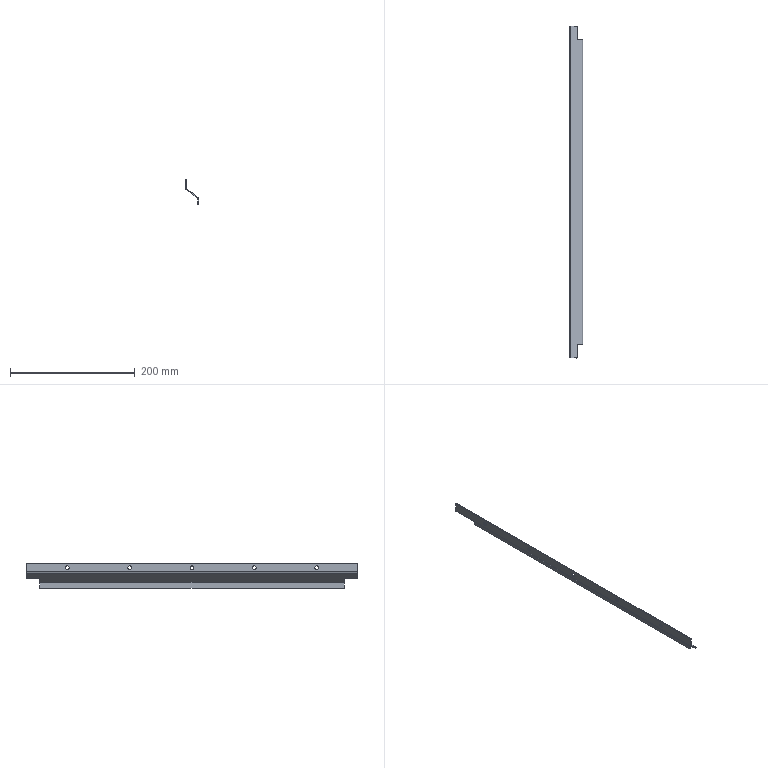Part | NX | features solid 2 | 1 solid | 28 faces | box 21.5 x 533 x 40 mm | volume 38151 mm3 | cylinder 14 | plane 14 | commonest cylinder face diameters 6 x12 3 x2
STEP:
#1=CARTESIAN_POINT('',(-1108.5,-824.5,202.25));
#2=VERTEX_POINT('',#1);
#3=CARTESIAN_POINT('',(-1107.,-824.5,202.25));
#4=VERTEX_POINT('',#3);
#5=CARTESIAN_POINT('',(-1641.931,-824.5,202.25));
#6=DIRECTION('',(1.,0.,0.));
#7=VECTOR('',#6,1000.);
#8=LINE('',#5,#7);
#9=EDGE_CURVE('',#2,#4,#8,.T.);
#10=ORIENTED_EDGE('',*,*,#9,.F.);
#11=CARTESIAN_POINT('',(-1108.5,-824.5,196.25));
#12=VERTEX_POINT('',#11);
#13=CARTESIAN_POINT('',(-1108.5,-824.5,199.25));
#14=DIRECTION('',(1.,0.,0.));
#15=DIRECTION('',(0.,0.,-1.));
#16=AXIS2_PLACEMENT_3D('',#13,#14,#15);
#17=CIRCLE('',#16,3.);
#18=EDGE_CURVE('',#12,#2,#17,.T.);
#19=ORIENTED_EDGE('',*,*,#18,.F.);
#20=CARTESIAN_POINT('',(-1107.,-824.5,196.25));
#21=VERTEX_POINT('',#20);
#22=CARTESIAN_POINT('',(-1641.931,-824.5,196.25));
#23=DIRECTION('',(1.,0.,0.));
#24=VECTOR('',#23,1000.);
#25=LINE('',#22,#24);
#26=EDGE_CURVE('',#21,#12,#25,.F.);
#27=ORIENTED_EDGE('',*,*,#26,.F.);
#28=CARTESIAN_POINT('',(-1107.,-824.5,199.25));
#29=DIRECTION('',(1.,0.,0.));
#30=DIRECTION('',(0.,1.,0.));
#31=AXIS2_PLACEMENT_3D('',#28,#29,#30);
#32=CIRCLE('',#31,3.);
#33=EDGE_CURVE('',#21,#4,#32,.T.);
#34=ORIENTED_EDGE('',*,*,#33,.T.);
#35=EDGE_LOOP('',(#10,#19,#27,#34));
#36=FACE_BOUND('',#35,.T.);
#37=CARTESIAN_POINT('',(-1641.931,-824.5,199.25));
#38=DIRECTION('',(1.,0.,0.));
#39=DIRECTION('',(0.,0.,-1.));
#40=AXIS2_PLACEMENT_3D('',#37,#38,#39);
#41=CYLINDRICAL_SURFACE('',#40,3.);
#42=ADVANCED_FACE('',(#36),#41,.F.);
#43=CARTESIAN_POINT('',(-1108.5,-924.5,202.25));
#44=VERTEX_POINT('',#43);
#45=CARTESIAN_POINT('',(-1107.,-924.5,202.25));
#46=VERTEX_POINT('',#45);
#47=CARTESIAN_POINT('',(-1641.931,-924.5,202.25));
#48=DIRECTION('',(1.,0.,0.));
#49=VECTOR('',#48,1000.);
#50=LINE('',#47,#49);
#51=EDGE_CURVE('',#44,#46,#50,.T.);
#52=ORIENTED_EDGE('',*,*,#51,.F.);
#53=CARTESIAN_POINT('',(-1108.5,-924.5,196.25));
#54=VERTEX_POINT('',#53);
#55=CARTESIAN_POINT('',(-1108.5,-924.5,199.25));
#56=DIRECTION('',(1.,0.,0.));
#57=DIRECTION('',(0.,0.,-1.));
#58=AXIS2_PLACEMENT_3D('',#55,#56,#57);
#59=CIRCLE('',#58,3.);
#60=EDGE_CURVE('',#54,#44,#59,.T.);
#61=ORIENTED_EDGE('',*,*,#60,.F.);
#62=CARTESIAN_POINT('',(-1107.,-924.5,196.25));
#63=VERTEX_POINT('',#62);
#64=CARTESIAN_POINT('',(-1641.931,-924.5,196.25));
#65=DIRECTION('',(1.,0.,0.));
#66=VECTOR('',#65,1000.);
#67=LINE('',#64,#66);
#68=EDGE_CURVE('',#63,#54,#67,.F.);
#69=ORIENTED_EDGE('',*,*,#68,.F.);
#70=CARTESIAN_POINT('',(-1107.,-924.5,199.25));
#71=DIRECTION('',(1.,0.,0.));
#72=DIRECTION('',(0.,1.,0.));
#73=AXIS2_PLACEMENT_3D('',#70,#71,#72);
#74=CIRCLE('',#73,3.);
#75=EDGE_CURVE('',#63,#46,#74,.T.);
#76=ORIENTED_EDGE('',*,*,#75,.T.);
#77=EDGE_LOOP('',(#52,#61,#69,#76));
#78=FACE_BOUND('',#77,.T.);
#79=CARTESIAN_POINT('',(-1641.931,-924.5,199.25));
#80=DIRECTION('',(1.,0.,0.));
#81=DIRECTION('',(0.,0.,-1.));
#82=AXIS2_PLACEMENT_3D('',#79,#80,#81);
#83=CYLINDRICAL_SURFACE('',#82,3.);
#84=ADVANCED_FACE('',(#78),#83,.F.);
#85=CARTESIAN_POINT('',(-1108.5,-1024.5,202.25));
#86=VERTEX_POINT('',#85);
#87=CARTESIAN_POINT('',(-1107.,-1024.5,202.25));
#88=VERTEX_POINT('',#87);
#89=CARTESIAN_POINT('',(-1641.931,-1024.5,202.25));
#90=DIRECTION('',(1.,0.,0.));
#91=VECTOR('',#90,1000.);
#92=LINE('',#89,#91);
#93=EDGE_CURVE('',#86,#88,#92,.T.);
#94=ORIENTED_EDGE('',*,*,#93,.F.);
#95=CARTESIAN_POINT('',(-1108.5,-1024.5,196.25));
#96=VERTEX_POINT('',#95);
#97=CARTESIAN_POINT('',(-1108.5,-1024.5,199.25));
#98=DIRECTION('',(1.,0.,0.));
#99=DIRECTION('',(0.,0.,-1.));
#100=AXIS2_PLACEMENT_3D('',#97,#98,#99);
#101=CIRCLE('',#100,3.);
#102=EDGE_CURVE('',#96,#86,#101,.T.);
#103=ORIENTED_EDGE('',*,*,#102,.F.);
#104=CARTESIAN_POINT('',(-1107.,-1024.5,196.25));
#105=VERTEX_POINT('',#104);
#106=CARTESIAN_POINT('',(-1641.931,-1024.5,196.25));
#107=DIRECTION('',(1.,0.,0.));
#108=VECTOR('',#107,1000.);
#109=LINE('',#106,#108);
#110=EDGE_CURVE('',#105,#96,#109,.F.);
#111=ORIENTED_EDGE('',*,*,#110,.F.);
#112=CARTESIAN_POINT('',(-1107.,-1024.5,199.25));
#113=DIRECTION('',(1.,0.,0.));
#114=DIRECTION('',(0.,1.,0.));
#115=AXIS2_PLACEMENT_3D('',#112,#113,#114);
#116=CIRCLE('',#115,3.);
#117=EDGE_CURVE('',#105,#88,#116,.T.);
#118=ORIENTED_EDGE('',*,*,#117,.T.);
#119=EDGE_LOOP('',(#94,#103,#111,#118));
#120=FACE_BOUND('',#119,.T.);
#121=CARTESIAN_POINT('',(-1641.931,-1024.5,199.25));
#122=DIRECTION('',(1.,0.,0.));
#123=DIRECTION('',(0.,0.,-1.));
#124=AXIS2_PLACEMENT_3D('',#121,#122,#123);
#125=CYLINDRICAL_SURFACE('',#124,3.);
#126=ADVANCED_FACE('',(#120),#125,.F.);
#127=CARTESIAN_POINT('',(-1107.,-1124.5,202.25));
#128=VERTEX_POINT('',#127);
#129=CARTESIAN_POINT('',(-1108.5,-1124.5,202.25));
#130=VERTEX_POINT('',#129);
#131=CARTESIAN_POINT('',(-1641.931,-1124.5,202.25));
#132=DIRECTION('',(1.,0.,0.));
#133=VECTOR('',#132,1000.);
#134=LINE('',#131,#133);
#135=EDGE_CURVE('',#128,#130,#134,.F.);
#136=ORIENTED_EDGE('',*,*,#135,.T.);
#137=CARTESIAN_POINT('',(-1108.5,-1124.5,196.25));
#138=VERTEX_POINT('',#137);
#139=CARTESIAN_POINT('',(-1108.5,-1124.5,199.25));
#140=DIRECTION('',(1.,0.,0.));
#141=DIRECTION('',(0.,0.,-1.));
#142=AXIS2_PLACEMENT_3D('',#139,#140,#141);
#143=CIRCLE('',#142,3.);
#144=EDGE_CURVE('',#138,#130,#143,.T.);
#145=ORIENTED_EDGE('',*,*,#144,.F.);
#146=CARTESIAN_POINT('',(-1107.,-1124.5,196.25));
#147=VERTEX_POINT('',#146);
#148=CARTESIAN_POINT('',(-1641.931,-1124.5,196.25));
#149=DIRECTION('',(1.,0.,0.));
#150=VECTOR('',#149,1000.);
#151=LINE('',#148,#150);
#152=EDGE_CURVE('',#138,#147,#151,.T.);
#153=ORIENTED_EDGE('',*,*,#152,.T.);
#154=CARTESIAN_POINT('',(-1107.,-1124.5,199.25));
#155=DIRECTION('',(1.,0.,0.));
#156=DIRECTION('',(0.,1.,0.));
#157=AXIS2_PLACEMENT_3D('',#154,#155,#156);
#158=CIRCLE('',#157,3.);
#159=EDGE_CURVE('',#147,#128,#158,.T.);
#160=ORIENTED_EDGE('',*,*,#159,.T.);
#161=EDGE_LOOP('',(#136,#145,#153,#160));
#162=FACE_BOUND('',#161,.T.);
#163=CARTESIAN_POINT('',(-1641.931,-1124.5,199.25));
#164=DIRECTION('',(1.,0.,0.));
#165=DIRECTION('',(0.,0.,-1.));
#166=AXIS2_PLACEMENT_3D('',#163,#164,#165);
#167=CYLINDRICAL_SURFACE('',#166,3.);
#168=ADVANCED_FACE('',(#162),#167,.F.);
#169=CARTESIAN_POINT('',(-1108.5,-1224.5,202.25));
#170=VERTEX_POINT('',#169);
#171=CARTESIAN_POINT('',(-1107.,-1224.5,202.25));
#172=VERTEX_POINT('',#171);
#173=CARTESIAN_POINT('',(-1641.931,-1224.5,202.25));
#174=DIRECTION('',(1.,0.,0.));
#175=VECTOR('',#174,1000.);
#176=LINE('',#173,#175);
#177=EDGE_CURVE('',#170,#172,#176,.T.);
#178=ORIENTED_EDGE('',*,*,#177,.F.);
#179=CARTESIAN_POINT('',(-1108.5,-1224.5,196.25));
#180=VERTEX_POINT('',#179);
#181=CARTESIAN_POINT('',(-1108.5,-1224.5,199.25));
#182=DIRECTION('',(1.,0.,0.));
#183=DIRECTION('',(0.,0.,-1.));
#184=AXIS2_PLACEMENT_3D('',#181,#182,#183);
#185=CIRCLE('',#184,3.);
#186=EDGE_CURVE('',#180,#170,#185,.T.);
#187=ORIENTED_EDGE('',*,*,#186,.F.);
#188=CARTESIAN_POINT('',(-1107.,-1224.5,196.25));
#189=VERTEX_POINT('',#188);
#190=CARTESIAN_POINT('',(-1641.931,-1224.5,196.25));
#191=DIRECTION('',(1.,0.,0.));
#192=VECTOR('',#191,1000.);
#193=LINE('',#190,#192);
#194=EDGE_CURVE('',#189,#180,#193,.F.);
#195=ORIENTED_EDGE('',*,*,#194,.F.);
#196=CARTESIAN_POINT('',(-1107.,-1224.5,199.25));
#197=DIRECTION('',(1.,0.,0.));
#198=DIRECTION('',(0.,1.,0.));
#199=AXIS2_PLACEMENT_3D('',#196,#197,#198);
#200=CIRCLE('',#199,3.);
#201=EDGE_CURVE('',#189,#172,#200,.T.);
#202=ORIENTED_EDGE('',*,*,#201,.T.);
#203=EDGE_LOOP('',(#178,#187,#195,#202));
#204=FACE_BOUND('',#203,.T.);
#205=CARTESIAN_POINT('',(-1641.931,-1224.5,199.25));
#206=DIRECTION('',(1.,0.,0.));
#207=DIRECTION('',(0.,0.,-1.));
#208=AXIS2_PLACEMENT_3D('',#205,#206,#207);
#209=CYLINDRICAL_SURFACE('',#208,3.);
#210=ADVANCED_FACE('',(#204),#209,.F.);
#211=CARTESIAN_POINT('',(-1088.5,-1269.,166.));
#212=VERTEX_POINT('',#211);
#213=CARTESIAN_POINT('',(-1087.,-1269.,166.));
#214=VERTEX_POINT('',#213);
#215=CARTESIAN_POINT('',(-1087.,-1269.,166.));
#216=DIRECTION('',(1.,0.,0.));
#217=VECTOR('',#216,1000.);
#218=LINE('',#215,#217);
#219=EDGE_CURVE('',#212,#214,#218,.T.);
#220=ORIENTED_EDGE('',*,*,#219,.T.);
#221=CARTESIAN_POINT('',(-1087.,-1269.,175.25));
#222=VERTEX_POINT('',#221);
#223=CARTESIAN_POINT('',(-1087.,-1269.,176.));
#224=DIRECTION('',(0.,0.,1.));
#225=VECTOR('',#224,1000.);
#226=LINE('',#223,#225);
#227=EDGE_CURVE('',#214,#222,#226,.T.);
#228=ORIENTED_EDGE('',*,*,#227,.T.);
#229=CARTESIAN_POINT('',(-1088.2,-1269.,177.65));
#230=VERTEX_POINT('',#229);
#231=CARTESIAN_POINT('',(-1090.,-1269.,175.25));
#232=DIRECTION('',(0.,-1.,0.));
#233=DIRECTION('',(0.,0.,-1.));
#234=AXIS2_PLACEMENT_3D('',#231,#232,#233);
#235=CIRCLE('',#234,3.);
#236=EDGE_CURVE('',#222,#230,#235,.T.);
#237=ORIENTED_EDGE('',*,*,#236,.T.);
#238=CARTESIAN_POINT('',(-1095.5,-1269.,183.125));
#239=VERTEX_POINT('',#238);
#240=CARTESIAN_POINT('',(-1107.6,-1269.,192.2));
#241=DIRECTION('',(-0.8,0.,0.6));
#242=VECTOR('',#241,1000.);
#243=LINE('',#240,#242);
#244=EDGE_CURVE('',#230,#239,#243,.T.);
#245=ORIENTED_EDGE('',*,*,#244,.T.);
#246=CARTESIAN_POINT('',(-1096.4,-1269.,181.925));
#247=VERTEX_POINT('',#246);
#248=CARTESIAN_POINT('',(-1095.5,-1269.,183.125));
#249=DIRECTION('',(0.6,0.,0.8));
#250=VECTOR('',#249,1000.);
#251=LINE('',#248,#250);
#252=EDGE_CURVE('',#247,#239,#251,.T.);
#253=ORIENTED_EDGE('',*,*,#252,.F.);
#254=CARTESIAN_POINT('',(-1089.1,-1269.,176.45));
#255=VERTEX_POINT('',#254);
#256=CARTESIAN_POINT('',(-1108.5,-1269.,191.));
#257=DIRECTION('',(-0.8,0.,0.6));
#258=VECTOR('',#257,1000.);
#259=LINE('',#256,#258);
#260=EDGE_CURVE('',#255,#247,#259,.T.);
#261=ORIENTED_EDGE('',*,*,#260,.F.);
#262=CARTESIAN_POINT('',(-1088.5,-1269.,175.25));
#263=VERTEX_POINT('',#262);
#264=CARTESIAN_POINT('',(-1090.,-1269.,175.25));
#265=DIRECTION('',(0.,-1.,0.));
#266=DIRECTION('',(0.,0.,-1.));
#267=AXIS2_PLACEMENT_3D('',#264,#265,#266);
#268=CIRCLE('',#267,1.5);
#269=EDGE_CURVE('',#263,#255,#268,.T.);
#270=ORIENTED_EDGE('',*,*,#269,.F.);
#271=CARTESIAN_POINT('',(-1088.5,-1269.,176.));
#272=DIRECTION('',(0.,0.,1.));
#273=VECTOR('',#272,1000.);
#274=LINE('',#271,#273);
#275=EDGE_CURVE('',#212,#263,#274,.T.);
#276=ORIENTED_EDGE('',*,*,#275,.F.);
#277=EDGE_LOOP('',(#220,#228,#237,#245,#253,#261,#270,#276));
#278=FACE_BOUND('',#277,.T.);
#279=CARTESIAN_POINT('',(-1087.,-1269.,176.));
#280=DIRECTION('',(0.,1.,0.));
#281=DIRECTION('',(1.,0.,0.));
#282=AXIS2_PLACEMENT_3D('',#279,#280,#281);
#283=PLANE('',#282);
#284=ADVANCED_FACE('',(#278),#283,.F.);
#285=ORIENTED_EDGE('',*,*,#252,.T.);
#286=CARTESIAN_POINT('',(-1095.5,-1291.,183.125));
#287=VERTEX_POINT('',#286);
#288=CARTESIAN_POINT('',(-1095.5,-1291.,183.125));
#289=DIRECTION('',(0.,-1.,0.));
#290=VECTOR('',#289,1000.);
#291=LINE('',#288,#290);
#292=EDGE_CURVE('',#239,#287,#291,.T.);
#293=ORIENTED_EDGE('',*,*,#292,.T.);
#294=CARTESIAN_POINT('',(-1096.4,-1291.,181.925));
#295=VERTEX_POINT('',#294);
#296=CARTESIAN_POINT('',(-1095.5,-1291.,183.125));
#297=DIRECTION('',(0.6,0.,0.8));
#298=VECTOR('',#297,1000.);
#299=LINE('',#296,#298);
#300=EDGE_CURVE('',#295,#287,#299,.T.);
#301=ORIENTED_EDGE('',*,*,#300,.F.);
#302=CARTESIAN_POINT('',(-1096.4,-1291.,181.925));
#303=DIRECTION('',(0.,-1.,0.));
#304=VECTOR('',#303,1000.);
#305=LINE('',#302,#304);
#306=EDGE_CURVE('',#247,#295,#305,.T.);
#307=ORIENTED_EDGE('',*,*,#306,.F.);
#308=EDGE_LOOP('',(#285,#293,#301,#307));
#309=FACE_BOUND('',#308,.T.);
#310=CARTESIAN_POINT('',(-1095.5,-1291.,183.125));
#311=DIRECTION('',(-0.8,0.,0.6));
#312=DIRECTION('',(0.,1.,0.));
#313=AXIS2_PLACEMENT_3D('',#310,#311,#312);
#314=PLANE('',#313);
#315=ADVANCED_FACE('',(#309),#314,.F.);
#316=CARTESIAN_POINT('',(-1088.5,-780.,175.25));
#317=VERTEX_POINT('',#316);
#318=CARTESIAN_POINT('',(-1088.5,-780.,166.));
#319=VERTEX_POINT('',#318);
#320=CARTESIAN_POINT('',(-1088.5,-780.,176.));
#321=DIRECTION('',(0.,0.,-1.));
#322=VECTOR('',#321,1000.);
#323=LINE('',#320,#322);
#324=EDGE_CURVE('',#317,#319,#323,.T.);
#325=ORIENTED_EDGE('',*,*,#324,.F.);
#326=CARTESIAN_POINT('',(-1089.1,-780.,176.45));
#327=VERTEX_POINT('',#326);
#328=CARTESIAN_POINT('',(-1090.,-780.,175.25));
#329=DIRECTION('',(0.,1.,0.));
#330=DIRECTION('',(0.,0.,-1.));
#331=AXIS2_PLACEMENT_3D('',#328,#329,#330);
#332=CIRCLE('',#331,1.5);
#333=EDGE_CURVE('',#327,#317,#332,.T.);
#334=ORIENTED_EDGE('',*,*,#333,.F.);
#335=CARTESIAN_POINT('',(-1096.4,-780.,181.925));
#336=VERTEX_POINT('',#335);
#337=CARTESIAN_POINT('',(-1108.5,-780.,191.));
#338=DIRECTION('',(0.8,0.,-0.6));
#339=VECTOR('',#338,1000.);
#340=LINE('',#337,#339);
#341=EDGE_CURVE('',#336,#327,#340,.T.);
#342=ORIENTED_EDGE('',*,*,#341,.F.);
#343=CARTESIAN_POINT('',(-1095.5,-780.,183.125));
#344=VERTEX_POINT('',#343);
#345=CARTESIAN_POINT('',(-1095.5,-780.,183.125));
#346=DIRECTION('',(0.6,0.,0.8));
#347=VECTOR('',#346,1000.);
#348=LINE('',#345,#347);
#349=EDGE_CURVE('',#336,#344,#348,.T.);
#350=ORIENTED_EDGE('',*,*,#349,.T.);
#351=CARTESIAN_POINT('',(-1088.2,-780.,177.65));
#352=VERTEX_POINT('',#351);
#353=CARTESIAN_POINT('',(-1107.6,-780.,192.2));
#354=DIRECTION('',(0.8,0.,-0.6));
#355=VECTOR('',#354,1000.);
#356=LINE('',#353,#355);
#357=EDGE_CURVE('',#344,#352,#356,.T.);
#358=ORIENTED_EDGE('',*,*,#357,.T.);
#359=CARTESIAN_POINT('',(-1087.,-780.,175.25));
#360=VERTEX_POINT('',#359);
#361=CARTESIAN_POINT('',(-1090.,-780.,175.25));
#362=DIRECTION('',(0.,1.,0.));
#363=DIRECTION('',(0.,0.,1.));
#364=AXIS2_PLACEMENT_3D('',#361,#362,#363);
#365=CIRCLE('',#364,3.);
#366=EDGE_CURVE('',#352,#360,#365,.T.);
#367=ORIENTED_EDGE('',*,*,#366,.T.);
#368=CARTESIAN_POINT('',(-1087.,-780.,166.));
#369=VERTEX_POINT('',#368);
#370=CARTESIAN_POINT('',(-1087.,-780.,176.));
#371=DIRECTION('',(0.,0.,-1.));
#372=VECTOR('',#371,1000.);
#373=LINE('',#370,#372);
#374=EDGE_CURVE('',#360,#369,#373,.T.);
#375=ORIENTED_EDGE('',*,*,#374,.T.);
#376=CARTESIAN_POINT('',(-1087.,-780.,166.));
#377=DIRECTION('',(1.,0.,0.));
#378=VECTOR('',#377,1000.);
#379=LINE('',#376,#378);
#380=EDGE_CURVE('',#319,#369,#379,.T.);
#381=ORIENTED_EDGE('',*,*,#380,.F.);
#382=EDGE_LOOP('',(#325,#334,#342,#350,#358,#367,#375,#381));
#383=FACE_BOUND('',#382,.T.);
#384=CARTESIAN_POINT('',(-1087.,-780.,176.));
#385=DIRECTION('',(0.,-1.,0.));
#386=DIRECTION('',(-1.,0.,0.));
#387=AXIS2_PLACEMENT_3D('',#384,#385,#386);
#388=PLANE('',#387);
#389=ADVANCED_FACE('',(#383),#388,.F.);
#390=CARTESIAN_POINT('',(-1096.4,-758.,181.925));
#391=VERTEX_POINT('',#390);
#392=CARTESIAN_POINT('',(-1095.5,-758.,183.125));
#393=VERTEX_POINT('',#392);
#394=CARTESIAN_POINT('',(-1095.5,-758.,183.125));
#395=DIRECTION('',(0.6,0.,0.8));
#396=VECTOR('',#395,1000.);
#397=LINE('',#394,#396);
#398=EDGE_CURVE('',#391,#393,#397,.T.);
#399=ORIENTED_EDGE('',*,*,#398,.T.);
#400=CARTESIAN_POINT('',(-1095.5,-1291.,183.125));
#401=DIRECTION('',(0.,-1.,0.));
#402=VECTOR('',#401,1000.);
#403=LINE('',#400,#402);
#404=EDGE_CURVE('',#393,#344,#403,.T.);
#405=ORIENTED_EDGE('',*,*,#404,.T.);
#406=ORIENTED_EDGE('',*,*,#349,.F.);
#407=CARTESIAN_POINT('',(-1096.4,-1291.,181.925));
#408=DIRECTION('',(0.,-1.,0.));
#409=VECTOR('',#408,1000.);
#410=LINE('',#407,#409);
#411=EDGE_CURVE('',#391,#336,#410,.T.);
#412=ORIENTED_EDGE('',*,*,#411,.F.);
#413=EDGE_LOOP('',(#399,#405,#406,#412));
#414=FACE_BOUND('',#413,.T.);
#415=CARTESIAN_POINT('',(-1095.5,-1291.,183.125));
#416=DIRECTION('',(-0.8,0.,0.6));
#417=DIRECTION('',(0.,1.,0.));
#418=AXIS2_PLACEMENT_3D('',#415,#416,#417);
#419=PLANE('',#418);
#420=ADVANCED_FACE('',(#414),#419,.F.);
#421=CARTESIAN_POINT('',(-1088.5,-1291.,166.));
#422=DIRECTION('',(0.,1.,0.));
#423=VECTOR('',#422,1000.);
#424=LINE('',#421,#423);
#425=EDGE_CURVE('',#212,#319,#424,.T.);
#426=ORIENTED_EDGE('',*,*,#425,.F.);
#427=ORIENTED_EDGE('',*,*,#275,.T.);
#428=CARTESIAN_POINT('',(-1088.5,-1291.,175.25));
#429=DIRECTION('',(0.,1.,0.));
#430=VECTOR('',#429,1000.);
#431=LINE('',#428,#430);
#432=EDGE_CURVE('',#263,#317,#431,.T.);
#433=ORIENTED_EDGE('',*,*,#432,.T.);
#434=ORIENTED_EDGE('',*,*,#324,.T.);
#435=EDGE_LOOP('',(#426,#427,#433,#434));
#436=FACE_BOUND('',#435,.T.);
#437=CARTESIAN_POINT('',(-1088.5,-1291.,176.));
#438=DIRECTION('',(1.,0.,0.));
#439=DIRECTION('',(0.,0.,-1.));
#440=AXIS2_PLACEMENT_3D('',#437,#438,#439);
#441=PLANE('',#440);
#442=ADVANCED_FACE('',(#436),#441,.F.);
#443=ORIENTED_EDGE('',*,*,#432,.F.);
#444=ORIENTED_EDGE('',*,*,#269,.T.);
#445=CARTESIAN_POINT('',(-1089.1,-1291.,176.45));
#446=DIRECTION('',(0.,1.,0.));
#447=VECTOR('',#446,1000.);
#448=LINE('',#445,#447);
#449=EDGE_CURVE('',#255,#327,#448,.T.);
#450=ORIENTED_EDGE('',*,*,#449,.T.);
#451=ORIENTED_EDGE('',*,*,#333,.T.);
#452=EDGE_LOOP('',(#443,#444,#450,#451));
#453=FACE_BOUND('',#452,.T.);
#454=CARTESIAN_POINT('',(-1090.,-1291.,175.25));
#455=DIRECTION('',(0.,1.,0.));
#456=DIRECTION('',(0.,0.,-1.));
#457=AXIS2_PLACEMENT_3D('',#454,#455,#456);
#458=CYLINDRICAL_SURFACE('',#457,1.5);
#459=ADVANCED_FACE('',(#453),#458,.F.);
#460=ORIENTED_EDGE('',*,*,#260,.T.);
#461=ORIENTED_EDGE('',*,*,#306,.T.);
#462=CARTESIAN_POINT('',(-1107.3,-1291.,190.1));
#463=VERTEX_POINT('',#462);
#464=CARTESIAN_POINT('',(-1108.5,-1291.,191.));
#465=DIRECTION('',(0.8,0.,-0.6));
#466=VECTOR('',#465,1000.);
#467=LINE('',#464,#466);
#468=EDGE_CURVE('',#463,#295,#467,.T.);
#469=ORIENTED_EDGE('',*,*,#468,.F.);
#470=CARTESIAN_POINT('',(-1107.3,-758.,190.1));
#471=VERTEX_POINT('',#470);
#472=CARTESIAN_POINT('',(-1107.3,-1291.,190.1));
#473=DIRECTION('',(0.,1.,0.));
#474=VECTOR('',#473,1000.);
#475=LINE('',#472,#474);
#476=EDGE_CURVE('',#463,#471,#475,.T.);
#477=ORIENTED_EDGE('',*,*,#476,.T.);
#478=CARTESIAN_POINT('',(-1108.5,-758.,191.));
#479=DIRECTION('',(0.8,0.,-0.6));
#480=VECTOR('',#479,1000.);
#481=LINE('',#478,#480);
#482=EDGE_CURVE('',#471,#391,#481,.T.);
#483=ORIENTED_EDGE('',*,*,#482,.T.);
#484=ORIENTED_EDGE('',*,*,#411,.T.);
#485=ORIENTED_EDGE('',*,*,#341,.T.);
#486=ORIENTED_EDGE('',*,*,#449,.F.);
#487=EDGE_LOOP('',(#460,#461,#469,#477,#483,#484,#485,#486));
#488=FACE_BOUND('',#487,.T.);
#489=CARTESIAN_POINT('',(-1108.5,-1291.,191.));
#490=DIRECTION('',(0.6,0.,0.8));
#491=DIRECTION('',(0.,-1.,0.));
#492=AXIS2_PLACEMENT_3D('',#489,#490,#491);
#493=PLANE('',#492);
#494=ADVANCED_FACE('',(#488),#493,.F.);
#495=CARTESIAN_POINT('',(-1108.5,-758.,192.5));
#496=VERTEX_POINT('',#495);
#497=CARTESIAN_POINT('',(-1105.5,-758.,192.5));
#498=DIRECTION('',(0.,-1.,0.));
#499=DIRECTION('',(0.,0.,-1.));
#500=AXIS2_PLACEMENT_3D('',#497,#498,#499);
#501=CIRCLE('',#500,3.);
#502=EDGE_CURVE('',#496,#471,#501,.T.);
#503=ORIENTED_EDGE('',*,*,#502,.T.);
#504=ORIENTED_EDGE('',*,*,#476,.F.);
#505=CARTESIAN_POINT('',(-1108.5,-1291.,192.5));
#506=VERTEX_POINT('',#505);
#507=CARTESIAN_POINT('',(-1105.5,-1291.,192.5));
#508=DIRECTION('',(0.,-1.,0.));
#509=DIRECTION('',(0.,0.,-1.));
#510=AXIS2_PLACEMENT_3D('',#507,#508,#509);
#511=CIRCLE('',#510,3.);
#512=EDGE_CURVE('',#506,#463,#511,.T.);
#513=ORIENTED_EDGE('',*,*,#512,.F.);
#514=CARTESIAN_POINT('',(-1108.5,-1291.,192.5));
#515=DIRECTION('',(0.,1.,0.));
#516=VECTOR('',#515,1000.);
#517=LINE('',#514,#516);
#518=EDGE_CURVE('',#506,#496,#517,.T.);
#519=ORIENTED_EDGE('',*,*,#518,.T.);
#520=EDGE_LOOP('',(#503,#504,#513,#519));
#521=FACE_BOUND('',#520,.T.);
#522=CARTESIAN_POINT('',(-1105.5,-1291.,192.5));
#523=DIRECTION('',(0.,1.,0.));
#524=DIRECTION('',(0.,0.,-1.));
#525=AXIS2_PLACEMENT_3D('',#522,#523,#524);
#526=CYLINDRICAL_SURFACE('',#525,3.);
#527=ADVANCED_FACE('',(#521),#526,.T.);
#528=ORIENTED_EDGE('',*,*,#186,.T.);
#529=CARTESIAN_POINT('',(-1108.5,-1224.5,199.25));
#530=DIRECTION('',(1.,0.,0.));
#531=DIRECTION('',(0.,0.,-1.));
#532=AXIS2_PLACEMENT_3D('',#529,#530,#531);
#533=CIRCLE('',#532,3.);
#534=EDGE_CURVE('',#170,#180,#533,.T.);
#535=ORIENTED_EDGE('',*,*,#534,.T.);
#536=EDGE_LOOP('',(#528,#535));
#537=FACE_BOUND('',#536,.T.);
#538=ORIENTED_EDGE('',*,*,#144,.T.);
#539=CARTESIAN_POINT('',(-1108.5,-1124.5,199.25));
#540=DIRECTION('',(1.,0.,0.));
#541=DIRECTION('',(0.,0.,-1.));
#542=AXIS2_PLACEMENT_3D('',#539,#540,#541);
#543=CIRCLE('',#542,3.);
#544=EDGE_CURVE('',#130,#138,#543,.T.);
#545=ORIENTED_EDGE('',*,*,#544,.T.);
#546=EDGE_LOOP('',(#538,#545));
#547=FACE_BOUND('',#546,.T.);
#548=ORIENTED_EDGE('',*,*,#102,.T.);
#549=CARTESIAN_POINT('',(-1108.5,-1024.5,199.25));
#550=DIRECTION('',(1.,0.,0.));
#551=DIRECTION('',(0.,0.,-1.));
#552=AXIS2_PLACEMENT_3D('',#549,#550,#551);
#553=CIRCLE('',#552,3.);
#554=EDGE_CURVE('',#86,#96,#553,.T.);
#555=ORIENTED_EDGE('',*,*,#554,.T.);
#556=EDGE_LOOP('',(#548,#555));
#557=FACE_BOUND('',#556,.T.);
#558=ORIENTED_EDGE('',*,*,#60,.T.);
#559=CARTESIAN_POINT('',(-1108.5,-924.5,199.25));
#560=DIRECTION('',(1.,0.,0.));
#561=DIRECTION('',(0.,0.,-1.));
#562=AXIS2_PLACEMENT_3D('',#559,#560,#561);
#563=CIRCLE('',#562,3.);
#564=EDGE_CURVE('',#44,#54,#563,.T.);
#565=ORIENTED_EDGE('',*,*,#564,.T.);
#566=EDGE_LOOP('',(#558,#565));
#567=FACE_BOUND('',#566,.T.);
#568=ORIENTED_EDGE('',*,*,#18,.T.);
#569=CARTESIAN_POINT('',(-1108.5,-824.5,199.25));
#570=DIRECTION('',(1.,0.,0.));
#571=DIRECTION('',(0.,0.,-1.));
#572=AXIS2_PLACEMENT_3D('',#569,#570,#571);
#573=CIRCLE('',#572,3.);
#574=EDGE_CURVE('',#2,#12,#573,.T.);
#575=ORIENTED_EDGE('',*,*,#574,.T.);
#576=EDGE_LOOP('',(#568,#575));
#577=FACE_BOUND('',#576,.T.);
#578=CARTESIAN_POINT('',(-1108.5,-758.,206.));
#579=VERTEX_POINT('',#578);
#580=CARTESIAN_POINT('',(-1108.5,-758.,191.));
#581=DIRECTION('',(0.,0.,-1.));
#582=VECTOR('',#581,1000.);
#583=LINE('',#580,#582);
#584=EDGE_CURVE('',#579,#496,#583,.T.);
#585=ORIENTED_EDGE('',*,*,#584,.T.);
#586=ORIENTED_EDGE('',*,*,#518,.F.);
#587=CARTESIAN_POINT('',(-1108.5,-1291.,206.));
#588=VERTEX_POINT('',#587);
#589=CARTESIAN_POINT('',(-1108.5,-1291.,191.));
#590=DIRECTION('',(0.,0.,-1.));
#591=VECTOR('',#590,1000.);
#592=LINE('',#589,#591);
#593=EDGE_CURVE('',#588,#506,#592,.T.);
#594=ORIENTED_EDGE('',*,*,#593,.F.);
#595=CARTESIAN_POINT('',(-1108.5,-1291.,206.));
#596=DIRECTION('',(0.,1.,0.));
#597=VECTOR('',#596,1000.);
#598=LINE('',#595,#597);
#599=EDGE_CURVE('',#588,#579,#598,.T.);
#600=ORIENTED_EDGE('',*,*,#599,.T.);
#601=EDGE_LOOP('',(#585,#586,#594,#600));
#602=FACE_BOUND('',#601,.T.);
#603=CARTESIAN_POINT('',(-1108.5,-1291.,191.));
#604=DIRECTION('',(1.,0.,0.));
#605=DIRECTION('',(0.,0.,-1.));
#606=AXIS2_PLACEMENT_3D('',#603,#604,#605);
#607=PLANE('',#606);
#608=ADVANCED_FACE('',(#537,#547,#557,#567,#577,#602),#607,.F.);
#609=ORIENTED_EDGE('',*,*,#227,.F.);
#610=CARTESIAN_POINT('',(-1087.,-1291.,166.));
#611=DIRECTION('',(0.,1.,0.));
#612=VECTOR('',#611,1000.);
#613=LINE('',#610,#612);
#614=EDGE_CURVE('',#214,#369,#613,.T.);
#615=ORIENTED_EDGE('',*,*,#614,.T.);
#616=ORIENTED_EDGE('',*,*,#374,.F.);
#617=CARTESIAN_POINT('',(-1087.,-1291.,175.25));
#618=DIRECTION('',(0.,1.,0.));
#619=VECTOR('',#618,1000.);
#620=LINE('',#617,#619);
#621=EDGE_CURVE('',#222,#360,#620,.T.);
#622=ORIENTED_EDGE('',*,*,#621,.F.);
#623=EDGE_LOOP('',(#609,#615,#616,#622));
#624=FACE_BOUND('',#623,.T.);
#625=CARTESIAN_POINT('',(-1087.,-1291.,176.));
#626=DIRECTION('',(1.,0.,0.));
#627=DIRECTION('',(0.,0.,-1.));
#628=AXIS2_PLACEMENT_3D('',#625,#626,#627);
#629=PLANE('',#628);
#630=ADVANCED_FACE('',(#624),#629,.T.);
#631=ORIENTED_EDGE('',*,*,#236,.F.);
#632=ORIENTED_EDGE('',*,*,#621,.T.);
#633=ORIENTED_EDGE('',*,*,#366,.F.);
#634=CARTESIAN_POINT('',(-1088.2,-1291.,177.65));
#635=DIRECTION('',(0.,1.,0.));
#636=VECTOR('',#635,1000.);
#637=LINE('',#634,#636);
#638=EDGE_CURVE('',#230,#352,#637,.T.);
#639=ORIENTED_EDGE('',*,*,#638,.F.);
#640=EDGE_LOOP('',(#631,#632,#633,#639));
#641=FACE_BOUND('',#640,.T.);
#642=CARTESIAN_POINT('',(-1090.,-1291.,175.25));
#643=DIRECTION('',(0.,1.,0.));
#644=DIRECTION('',(0.,0.,-1.));
#645=AXIS2_PLACEMENT_3D('',#642,#643,#644);
#646=CYLINDRICAL_SURFACE('',#645,3.);
#647=ADVANCED_FACE('',(#641),#646,.T.);
#648=ORIENTED_EDGE('',*,*,#292,.F.);
#649=ORIENTED_EDGE('',*,*,#244,.F.);
#650=ORIENTED_EDGE('',*,*,#638,.T.);
#651=ORIENTED_EDGE('',*,*,#357,.F.);
#652=ORIENTED_EDGE('',*,*,#404,.F.);
#653=CARTESIAN_POINT('',(-1106.4,-758.,191.3));
#654=VERTEX_POINT('',#653);
#655=CARTESIAN_POINT('',(-1107.6,-758.,192.2));
#656=DIRECTION('',(0.8,0.,-0.6));
#657=VECTOR('',#656,1000.);
#658=LINE('',#655,#657);
#659=EDGE_CURVE('',#654,#393,#658,.T.);
#660=ORIENTED_EDGE('',*,*,#659,.F.);
#661=CARTESIAN_POINT('',(-1106.4,-1291.,191.3));
#662=VERTEX_POINT('',#661);
#663=CARTESIAN_POINT('',(-1106.4,-1291.,191.3));
#664=DIRECTION('',(0.,1.,0.));
#665=VECTOR('',#664,1000.);
#666=LINE('',#663,#665);
#667=EDGE_CURVE('',#662,#654,#666,.T.);
#668=ORIENTED_EDGE('',*,*,#667,.F.);
#669=CARTESIAN_POINT('',(-1107.6,-1291.,192.2));
#670=DIRECTION('',(0.8,0.,-0.6));
#671=VECTOR('',#670,1000.);
#672=LINE('',#669,#671);
#673=EDGE_CURVE('',#662,#287,#672,.T.);
#674=ORIENTED_EDGE('',*,*,#673,.T.);
#675=EDGE_LOOP('',(#648,#649,#650,#651,#652,#660,#668,#674));
#676=FACE_BOUND('',#675,.T.);
#677=CARTESIAN_POINT('',(-1107.6,-1291.,192.2));
#678=DIRECTION('',(0.6,0.,0.8));
#679=DIRECTION('',(0.,-1.,0.));
#680=AXIS2_PLACEMENT_3D('',#677,#678,#679);
#681=PLANE('',#680);
#682=ADVANCED_FACE('',(#676),#681,.T.);
#683=CARTESIAN_POINT('',(-1107.,-758.,192.5));
#684=VERTEX_POINT('',#683);
#685=CARTESIAN_POINT('',(-1105.5,-758.,192.5));
#686=DIRECTION('',(0.,-1.,0.));
#687=DIRECTION('',(0.,0.,-1.));
#688=AXIS2_PLACEMENT_3D('',#685,#686,#687);
#689=CIRCLE('',#688,1.5);
#690=EDGE_CURVE('',#684,#654,#689,.T.);
#691=ORIENTED_EDGE('',*,*,#690,.F.);
#692=CARTESIAN_POINT('',(-1107.,-1291.,192.5));
#693=VERTEX_POINT('',#692);
#694=CARTESIAN_POINT('',(-1107.,-1291.,192.5));
#695=DIRECTION('',(0.,1.,0.));
#696=VECTOR('',#695,1000.);
#697=LINE('',#694,#696);
#698=EDGE_CURVE('',#693,#684,#697,.T.);
#699=ORIENTED_EDGE('',*,*,#698,.F.);
#700=CARTESIAN_POINT('',(-1105.5,-1291.,192.5));
#701=DIRECTION('',(0.,-1.,0.));
#702=DIRECTION('',(0.,0.,-1.));
#703=AXIS2_PLACEMENT_3D('',#700,#701,#702);
#704=CIRCLE('',#703,1.5);
#705=EDGE_CURVE('',#693,#662,#704,.T.);
#706=ORIENTED_EDGE('',*,*,#705,.T.);
#707=ORIENTED_EDGE('',*,*,#667,.T.);
#708=EDGE_LOOP('',(#691,#699,#706,#707));
#709=FACE_BOUND('',#708,.T.);
#710=CARTESIAN_POINT('',(-1105.5,-1291.,192.5));
#711=DIRECTION('',(0.,1.,0.));
#712=DIRECTION('',(0.,0.,-1.));
#713=AXIS2_PLACEMENT_3D('',#710,#711,#712);
#714=CYLINDRICAL_SURFACE('',#713,1.5);
#715=ADVANCED_FACE('',(#709),#714,.F.);
#716=ORIENTED_EDGE('',*,*,#201,.F.);
#717=CARTESIAN_POINT('',(-1107.,-1224.5,199.25));
#718=DIRECTION('',(1.,0.,0.));
#719=DIRECTION('',(0.,1.,0.));
#720=AXIS2_PLACEMENT_3D('',#717,#718,#719);
#721=CIRCLE('',#720,3.);
#722=EDGE_CURVE('',#172,#189,#721,.T.);
#723=ORIENTED_EDGE('',*,*,#722,.F.);
#724=EDGE_LOOP('',(#716,#723));
#725=FACE_BOUND('',#724,.T.);
#726=ORIENTED_EDGE('',*,*,#159,.F.);
#727=CARTESIAN_POINT('',(-1107.,-1124.5,199.25));
#728=DIRECTION('',(1.,0.,0.));
#729=DIRECTION('',(0.,1.,0.));
#730=AXIS2_PLACEMENT_3D('',#727,#728,#729);
#731=CIRCLE('',#730,3.);
#732=EDGE_CURVE('',#128,#147,#731,.T.);
#733=ORIENTED_EDGE('',*,*,#732,.F.);
#734=EDGE_LOOP('',(#726,#733));
#735=FACE_BOUND('',#734,.T.);
#736=ORIENTED_EDGE('',*,*,#117,.F.);
#737=CARTESIAN_POINT('',(-1107.,-1024.5,199.25));
#738=DIRECTION('',(1.,0.,0.));
#739=DIRECTION('',(0.,1.,0.));
#740=AXIS2_PLACEMENT_3D('',#737,#738,#739);
#741=CIRCLE('',#740,3.);
#742=EDGE_CURVE('',#88,#105,#741,.T.);
#743=ORIENTED_EDGE('',*,*,#742,.F.);
#744=EDGE_LOOP('',(#736,#743));
#745=FACE_BOUND('',#744,.T.);
#746=ORIENTED_EDGE('',*,*,#75,.F.);
#747=CARTESIAN_POINT('',(-1107.,-924.5,199.25));
#748=DIRECTION('',(1.,0.,0.));
#749=DIRECTION('',(0.,1.,0.));
#750=AXIS2_PLACEMENT_3D('',#747,#748,#749);
#751=CIRCLE('',#750,3.);
#752=EDGE_CURVE('',#46,#63,#751,.T.);
#753=ORIENTED_EDGE('',*,*,#752,.F.);
#754=EDGE_LOOP('',(#746,#753));
#755=FACE_BOUND('',#754,.T.);
#756=ORIENTED_EDGE('',*,*,#33,.F.);
#757=CARTESIAN_POINT('',(-1107.,-824.5,199.25));
#758=DIRECTION('',(1.,0.,0.));
#759=DIRECTION('',(0.,1.,0.));
#760=AXIS2_PLACEMENT_3D('',#757,#758,#759);
#761=CIRCLE('',#760,3.);
#762=EDGE_CURVE('',#4,#21,#761,.T.);
#763=ORIENTED_EDGE('',*,*,#762,.F.);
#764=EDGE_LOOP('',(#756,#763));
#765=FACE_BOUND('',#764,.T.);
#766=CARTESIAN_POINT('',(-1107.,-758.,206.));
#767=VERTEX_POINT('',#766);
#768=CARTESIAN_POINT('',(-1107.,-758.,191.));
#769=DIRECTION('',(0.,0.,-1.));
#770=VECTOR('',#769,1000.);
#771=LINE('',#768,#770);
#772=EDGE_CURVE('',#767,#684,#771,.T.);
#773=ORIENTED_EDGE('',*,*,#772,.F.);
#774=CARTESIAN_POINT('',(-1107.,-1291.,206.));
#775=VERTEX_POINT('',#774);
#776=CARTESIAN_POINT('',(-1107.,-1291.,206.));
#777=DIRECTION('',(0.,1.,0.));
#778=VECTOR('',#777,1000.);
#779=LINE('',#776,#778);
#780=EDGE_CURVE('',#775,#767,#779,.T.);
#781=ORIENTED_EDGE('',*,*,#780,.F.);
#782=CARTESIAN_POINT('',(-1107.,-1291.,191.));
#783=DIRECTION('',(0.,0.,-1.));
#784=VECTOR('',#783,1000.);
#785=LINE('',#782,#784);
#786=EDGE_CURVE('',#775,#693,#785,.T.);
#787=ORIENTED_EDGE('',*,*,#786,.T.);
#788=ORIENTED_EDGE('',*,*,#698,.T.);
#789=EDGE_LOOP('',(#773,#781,#787,#788));
#790=FACE_BOUND('',#789,.T.);
#791=CARTESIAN_POINT('',(-1107.,-1291.,191.));
#792=DIRECTION('',(1.,0.,0.));
#793=DIRECTION('',(0.,0.,-1.));
#794=AXIS2_PLACEMENT_3D('',#791,#792,#793);
#795=PLANE('',#794);
#796=ADVANCED_FACE('',(#725,#735,#745,#755,#765,#790),#795,.T.);
#797=ORIENTED_EDGE('',*,*,#599,.F.);
#798=CARTESIAN_POINT('',(-1108.5,-1291.,206.));
#799=DIRECTION('',(1.,0.,0.));
#800=VECTOR('',#799,1000.);
#801=LINE('',#798,#800);
#802=EDGE_CURVE('',#588,#775,#801,.T.);
#803=ORIENTED_EDGE('',*,*,#802,.T.);
#804=ORIENTED_EDGE('',*,*,#780,.T.);
#805=CARTESIAN_POINT('',(-1108.5,-758.,206.));
#806=DIRECTION('',(1.,0.,0.));
#807=VECTOR('',#806,1000.);
#808=LINE('',#805,#807);
#809=EDGE_CURVE('',#579,#767,#808,.T.);
#810=ORIENTED_EDGE('',*,*,#809,.F.);
#811=EDGE_LOOP('',(#797,#803,#804,#810));
#812=FACE_BOUND('',#811,.T.);
#813=CARTESIAN_POINT('',(-1108.5,-1291.,206.));
#814=DIRECTION('',(0.,0.,-1.));
#815=DIRECTION('',(-1.,0.,0.));
#816=AXIS2_PLACEMENT_3D('',#813,#814,#815);
#817=PLANE('',#816);
#818=ADVANCED_FACE('',(#812),#817,.F.);
#819=ORIENTED_EDGE('',*,*,#398,.F.);
#820=ORIENTED_EDGE('',*,*,#482,.F.);
#821=ORIENTED_EDGE('',*,*,#502,.F.);
#822=ORIENTED_EDGE('',*,*,#584,.F.);
#823=ORIENTED_EDGE('',*,*,#809,.T.);
#824=ORIENTED_EDGE('',*,*,#772,.T.);
#825=ORIENTED_EDGE('',*,*,#690,.T.);
#826=ORIENTED_EDGE('',*,*,#659,.T.);
#827=EDGE_LOOP('',(#819,#820,#821,#822,#823,#824,#825,#826));
#828=FACE_BOUND('',#827,.T.);
#829=CARTESIAN_POINT('',(-1108.5,-758.,191.));
#830=DIRECTION('',(0.,-1.,0.));
#831=DIRECTION('',(-1.,0.,0.));
#832=AXIS2_PLACEMENT_3D('',#829,#830,#831);
#833=PLANE('',#832);
#834=ADVANCED_FACE('',(#828),#833,.F.);
#835=ORIENTED_EDGE('',*,*,#219,.F.);
#836=ORIENTED_EDGE('',*,*,#425,.T.);
#837=ORIENTED_EDGE('',*,*,#380,.T.);
#838=ORIENTED_EDGE('',*,*,#614,.F.);
#839=EDGE_LOOP('',(#835,#836,#837,#838));
#840=FACE_BOUND('',#839,.T.);
#841=CARTESIAN_POINT('',(-1088.5,-1291.,166.));
#842=DIRECTION('',(0.,0.,-1.));
#843=DIRECTION('',(-1.,0.,0.));
#844=AXIS2_PLACEMENT_3D('',#841,#842,#843);
#845=PLANE('',#844);
#846=ADVANCED_FACE('',(#840),#845,.T.);
#847=ORIENTED_EDGE('',*,*,#468,.T.);
#848=ORIENTED_EDGE('',*,*,#300,.T.);
#849=ORIENTED_EDGE('',*,*,#673,.F.);
#850=ORIENTED_EDGE('',*,*,#705,.F.);
#851=ORIENTED_EDGE('',*,*,#786,.F.);
#852=ORIENTED_EDGE('',*,*,#802,.F.);
#853=ORIENTED_EDGE('',*,*,#593,.T.);
#854=ORIENTED_EDGE('',*,*,#512,.T.);
#855=EDGE_LOOP('',(#847,#848,#849,#850,#851,#852,#853,#854));
#856=FACE_BOUND('',#855,.T.);
#857=CARTESIAN_POINT('',(-1088.5,-1291.,176.));
#858=DIRECTION('',(0.,-1.,0.));
#859=DIRECTION('',(-1.,0.,0.));
#860=AXIS2_PLACEMENT_3D('',#857,#858,#859);
#861=PLANE('',#860);
#862=ADVANCED_FACE('',(#856),#861,.T.);
#863=ORIENTED_EDGE('',*,*,#534,.F.);
#864=ORIENTED_EDGE('',*,*,#177,.T.);
#865=ORIENTED_EDGE('',*,*,#722,.T.);
#866=ORIENTED_EDGE('',*,*,#194,.T.);
#867=EDGE_LOOP('',(#863,#864,#865,#866));
#868=FACE_BOUND('',#867,.T.);
#869=CARTESIAN_POINT('',(-1641.931,-1224.5,199.25));
#870=DIRECTION('',(1.,0.,0.));
#871=DIRECTION('',(0.,0.,-1.));
#872=AXIS2_PLACEMENT_3D('',#869,#870,#871);
#873=CYLINDRICAL_SURFACE('',#872,3.);
#874=ADVANCED_FACE('',(#868),#873,.F.);
#875=ORIENTED_EDGE('',*,*,#544,.F.);
#876=ORIENTED_EDGE('',*,*,#135,.F.);
#877=ORIENTED_EDGE('',*,*,#732,.T.);
#878=ORIENTED_EDGE('',*,*,#152,.F.);
#879=EDGE_LOOP('',(#875,#876,#877,#878));
#880=FACE_BOUND('',#879,.T.);
#881=CARTESIAN_POINT('',(-1641.931,-1124.5,199.25));
#882=DIRECTION('',(1.,0.,0.));
#883=DIRECTION('',(0.,0.,-1.));
#884=AXIS2_PLACEMENT_3D('',#881,#882,#883);
#885=CYLINDRICAL_SURFACE('',#884,3.);
#886=ADVANCED_FACE('',(#880),#885,.F.);
#887=ORIENTED_EDGE('',*,*,#554,.F.);
#888=ORIENTED_EDGE('',*,*,#93,.T.);
#889=ORIENTED_EDGE('',*,*,#742,.T.);
#890=ORIENTED_EDGE('',*,*,#110,.T.);
#891=EDGE_LOOP('',(#887,#888,#889,#890));
#892=FACE_BOUND('',#891,.T.);
#893=CARTESIAN_POINT('',(-1641.931,-1024.5,199.25));
#894=DIRECTION('',(1.,0.,0.));
#895=DIRECTION('',(0.,0.,-1.));
#896=AXIS2_PLACEMENT_3D('',#893,#894,#895);
#897=CYLINDRICAL_SURFACE('',#896,3.);
#898=ADVANCED_FACE('',(#892),#897,.F.);
#899=ORIENTED_EDGE('',*,*,#564,.F.);
#900=ORIENTED_EDGE('',*,*,#51,.T.);
#901=ORIENTED_EDGE('',*,*,#752,.T.);
#902=ORIENTED_EDGE('',*,*,#68,.T.);
#903=EDGE_LOOP('',(#899,#900,#901,#902));
#904=FACE_BOUND('',#903,.T.);
#905=CARTESIAN_POINT('',(-1641.931,-924.5,199.25));
#906=DIRECTION('',(1.,0.,0.));
#907=DIRECTION('',(0.,0.,-1.));
#908=AXIS2_PLACEMENT_3D('',#905,#906,#907);
#909=CYLINDRICAL_SURFACE('',#908,3.);
#910=ADVANCED_FACE('',(#904),#909,.F.);
#911=ORIENTED_EDGE('',*,*,#574,.F.);
#912=ORIENTED_EDGE('',*,*,#9,.T.);
#913=ORIENTED_EDGE('',*,*,#762,.T.);
#914=ORIENTED_EDGE('',*,*,#26,.T.);
#915=EDGE_LOOP('',(#911,#912,#913,#914));
#916=FACE_BOUND('',#915,.T.);
#917=CARTESIAN_POINT('',(-1641.931,-824.5,199.25));
#918=DIRECTION('',(1.,0.,0.));
#919=DIRECTION('',(0.,0.,-1.));
#920=AXIS2_PLACEMENT_3D('',#917,#918,#919);
#921=CYLINDRICAL_SURFACE('',#920,3.);
#922=ADVANCED_FACE('',(#916),#921,.F.);
#923=CLOSED_SHELL('',(#42,#84,#126,#168,#210,#284,#315,#389,#420,#442,#459,#494,#527,#608,#630,#647,#682,#715,#796,#818,#834,#846,#862,#874,#886,#898,#910,#922));
#924=MANIFOLD_SOLID_BREP('',#923);
#925=(LENGTH_UNIT()NAMED_UNIT(*)SI_UNIT(.MILLI.,.METRE.));
#926=UNCERTAINTY_MEASURE_WITH_UNIT(LENGTH_MEASURE(0.00001),#925,'','');
#927=(NAMED_UNIT(*)PLANE_ANGLE_UNIT()SI_UNIT($,.RADIAN.));
#928=(NAMED_UNIT(*)SI_UNIT($,.STERADIAN.)SOLID_ANGLE_UNIT());
#929=(GEOMETRIC_REPRESENTATION_CONTEXT(3)GLOBAL_UNCERTAINTY_ASSIGNED_CONTEXT((#926))GLOBAL_UNIT_ASSIGNED_CONTEXT((#925,#927,#928))REPRESENTATION_CONTEXT('',''));
#930=ADVANCED_BREP_SHAPE_REPRESENTATION('',(#924),#929);